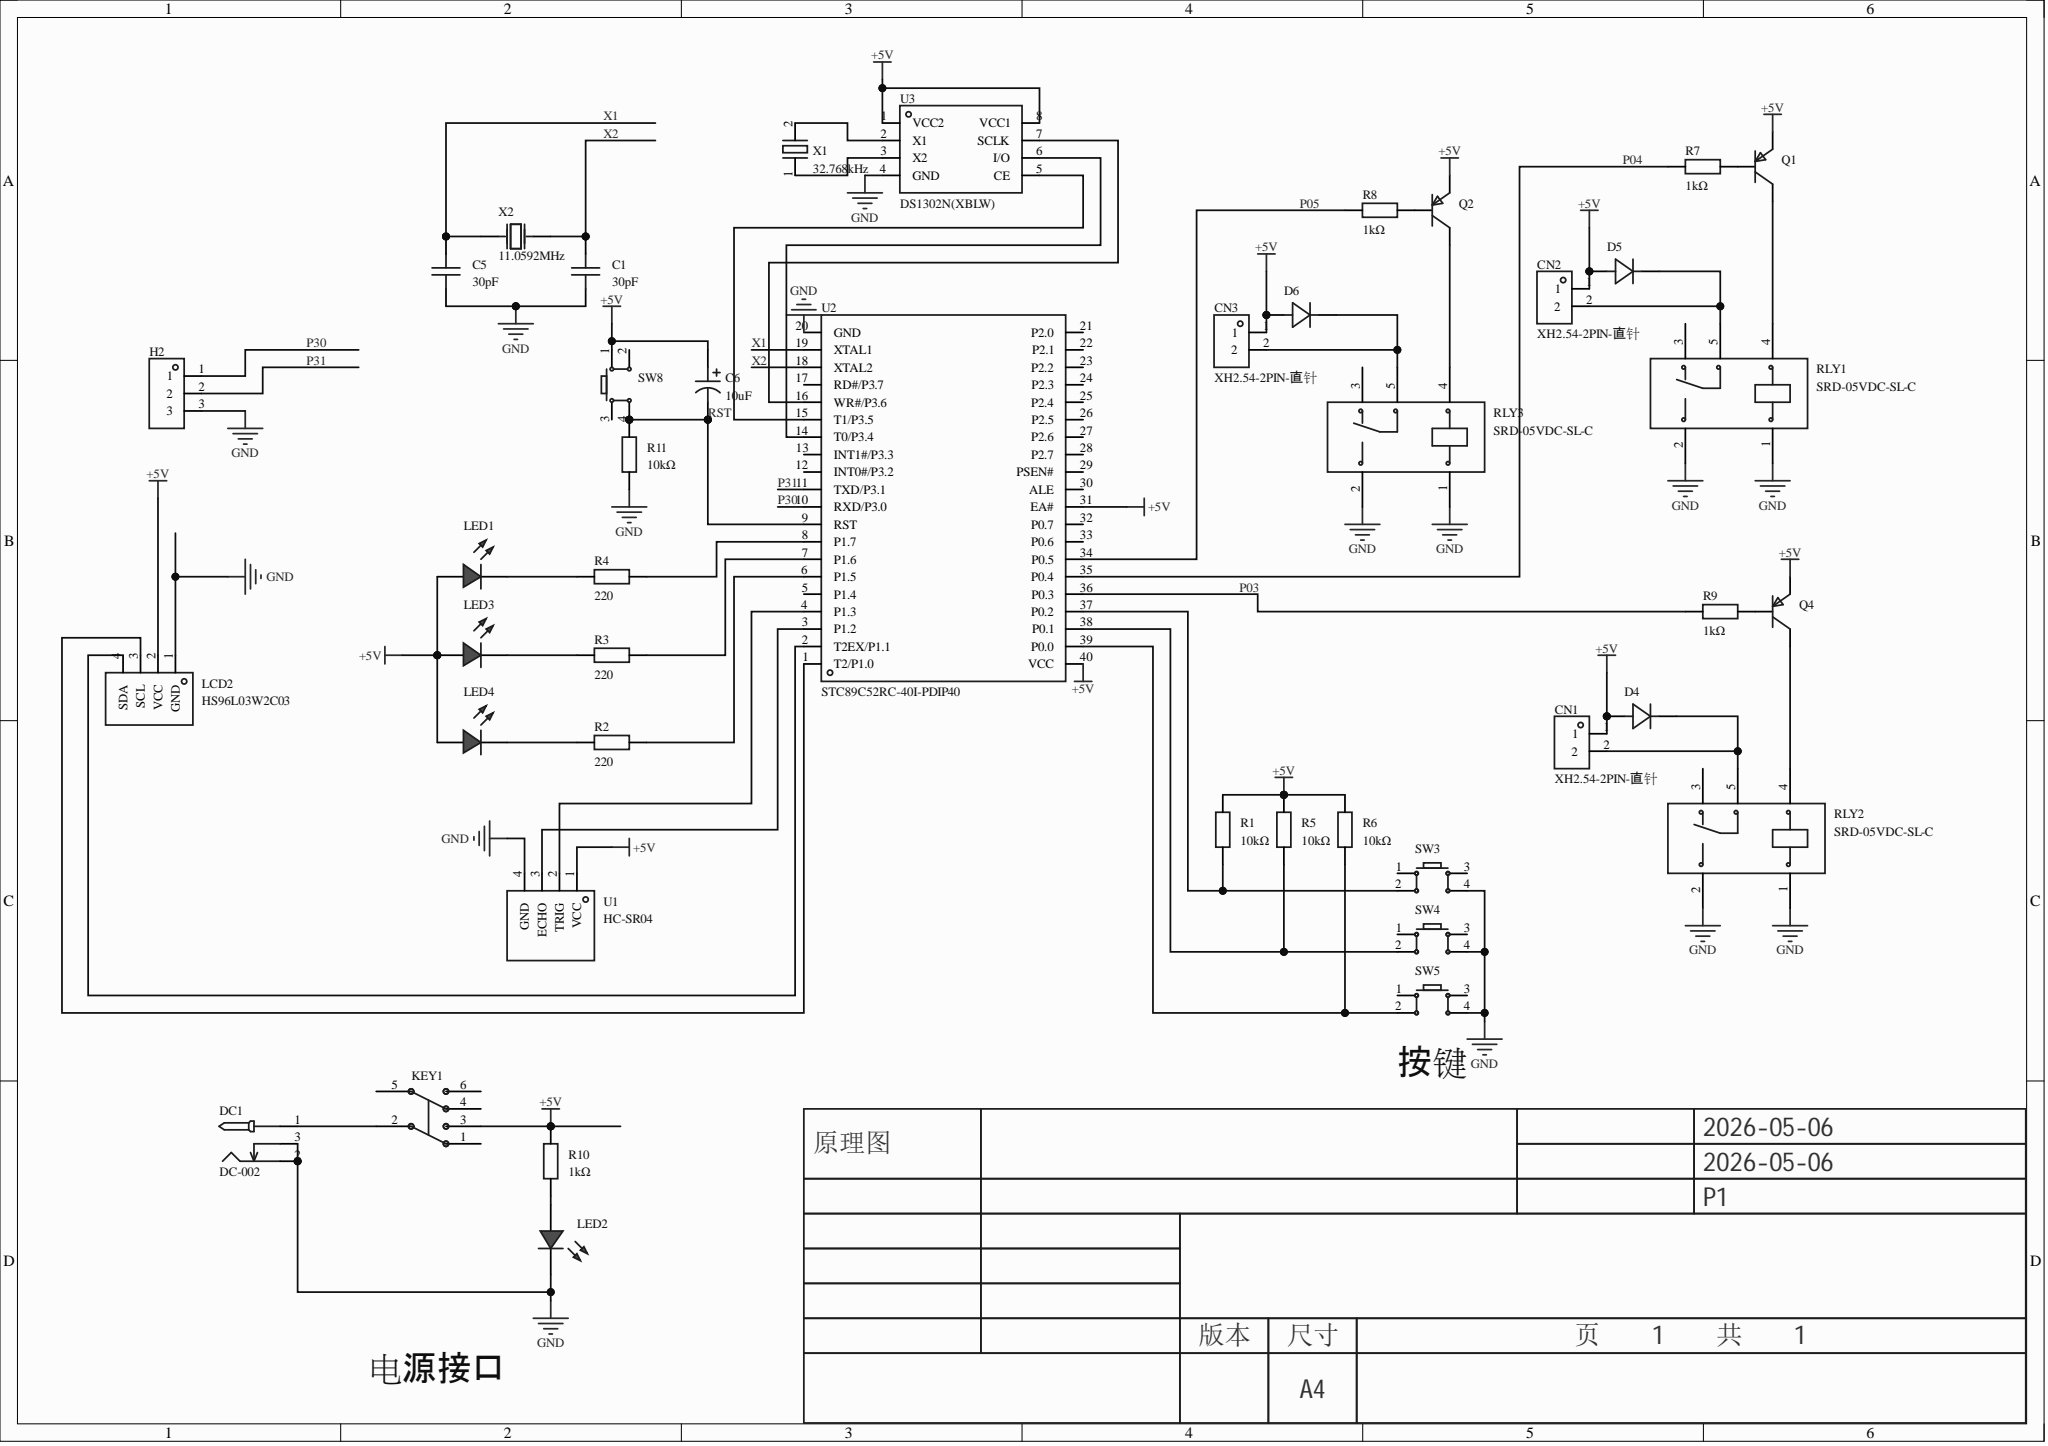Circuit board | Altium Designer | 43 parts | 39 nets
Bill of materials:
Comment,Description,Designator,Footprint,LibRef,Quantity
"30pF","","C1, C5","CAP-TH_L3.8-W2.5-P2.54-D0.50","C315C300K3G5TA7301","2"
"10uF","","C6","CAP-TH_BD5.0-P2.00-D0.8-FD-10UF50VC110GL","10UF50VC110GL","1"
"XH2.54-2PIN-直针","","CN1, CN2, CN3","CONN-TH_XH2.54-2P","XH2.54-2PIN-直针","3"
"","","D4, D5, D6","DO_1N4007","D_1N4007A","3"
"DC-002","","DC1","DC-IN-TH_DC-3510","DC-002","1"
"","","H2","HDR-TH_3P-P2.54-V-M","HDR-M_2.54_1x3P","1"
"无自锁开关 8.5×8.5 无声","","KEY1","SW-TH_6P-L8.5-W8.5-P2.54","无自锁开关 8.5×8.5 无声","1"
"HS96L03W2C03","","LCD2","OLED-TH_L27.8-W27.2-P2.54_C9900033791","HS96L03W2C03","1"
"","","LED1, LED2, LED3, LED4","LED_TH-3mm","LED_TH-R_3mm","4"
"","","Q1, Q2, Q4","S8550P_TO-92","S8550_TO_PNP","3"
"10kΩ","","R1, R5, R6, R11","Res_1/8W","Res_AXIAL-1/8W","4"
"220","","R2, R3, R4","R0603","Res_0603","3"
"1kΩ","","R7, R8, R9, R10","Res_1/8W","Res_AXIAL-1/8W","4"
"SRD-05VDC-SL-C","","RLY1, RLY2, RLY3","RELAY-TH_SRD-XXVDC-XL-C","SRD-05VDC-SL-C","3"
"","","SW3, SW4, SW5, SW8","SW-TH_4P-L6.0-W6.0-P4.50-LS6.5","Key_TH_6x6x6","4"
"HC-SR04","","U1","TH_HC-SR04V","HC-SR04","1"
"STC89C52RC-40I-PDIP40","","U2","DIP-40_L52.0-W13.7-P2.54-LS15.2-BL","STC89C52RC-40I-PDIP40","1"
"DS1302N(XBLW)","","U3","PDIP-8_L9.3-W6.4-P2.54-LS7.6-BL","DS1302N(XBLW)","1"
"32.768kHz","","X1","CRYSTAL-TH_BD1.4-P0.45-D0.2","AB15T-32.768KHZ","1"
"11.059MHz","","X2","OSC-TH_L11.1-W4.7-P4.88","9AC11059302060C3","1"
Netlist (Protel format):
[
C1
CAP-TH_L3.8-W2.5-P2.54-D0.50
30pF



]
[
C5
CAP-TH_L3.8-W2.5-P2.54-D0.50
30pF



]
[
C6
CAP-TH_BD5.0-P2.00-D0.8-FD-10UF50VC110GL
10uF



]
[
CN1
CONN-TH_XH2.54-2P
XH2.54-2PIN-直针



]
[
CN2
CONN-TH_XH2.54-2P
XH2.54-2PIN-直针



]
[
CN3
CONN-TH_XH2.54-2P
XH2.54-2PIN-直针



]
[
D4
DO_1N4007




]
[
D5
DO_1N4007




]
[
D6
DO_1N4007




]
[
DC1
DC-IN-TH_DC-3510
DC-002



]
[
H2
HDR-TH_3P-P2.54-V-M




]
[
KEY1
SW-TH_6P-L8.5-W8.5-P2.54
无自锁开关 8.5×8.5 无声



]
[
LCD2
OLED-TH_L27.8-W27.2-P2.54_C9900033791
HS96L03W2C03



]
[
LED1
LED_TH-3mm




]
[
LED2
LED_TH-3mm




]
[
LED3
LED_TH-3mm




]
[
LED4
LED_TH-3mm




]
[
Q1
S8550P_TO-92




]
[
Q2
S8550P_TO-92




]
[
Q4
S8550P_TO-92




]
[
R1
Res_1/8W
10kΩ



]
[
R2
R0603
220



]
[
R3
R0603
220



]
[
R4
R0603
220



]
[
R5
Res_1/8W
10kΩ



]
[
R6
Res_1/8W
10kΩ



]
[
R7
Res_1/8W
1kΩ



]
[
R8
Res_1/8W
1kΩ



]
[
R9
Res_1/8W
1kΩ



]
[
R10
Res_1/8W
1kΩ



]
[
R11
Res_1/8W
10kΩ



]
[
RLY1
RELAY-TH_SRD-XXVDC-XL-C
SRD-05VDC-SL-C



]
[
RLY2
RELAY-TH_SRD-XXVDC-XL-C
SRD-05VDC-SL-C



]
[
RLY3
RELAY-TH_SRD-XXVDC-XL-C
SRD-05VDC-SL-C



]
[
SW3
SW-TH_4P-L6.0-W6.0-P4.50-LS6.5




]
[
SW4
SW-TH_4P-L6.0-W6.0-P4.50-LS6.5




]
[
SW5
SW-TH_4P-L6.0-W6.0-P4.50-LS6.5




]
[
SW8
SW-TH_4P-L6.0-W6.0-P4.50-LS6.5




]
[
U1
TH_HC-SR04V
HC-SR04



]
[
U2
DIP-40_L52.0-W13.7-P2.54-LS15.2-BL
STC89C52RC-40I-PDIP40



]
[
U3
PDIP-8_L9.3-W6.4-P2.54-LS7.6-BL
DS1302N(XBLW)



]
[
X1
CRYSTAL-TH_BD1.4-P0.45-D0.2
32.768kHz



]
[
X2
OSC-TH_L11.1-W4.7-P4.88
11.0592MHz



]
(
X2
C1-2
U2-18
X2-2
)
(
X1
C5-2
U2-19
X2-1
)
(
RST
C6-2
R11-2
SW8-4
U2-9
)
(
P31
H2-2
U2-11
)
(
P30
H2-1
U2-10
)
(
P05
R8-2
U2-34
)
(
P04
R7-2
U2-35
)
(
P03
R9-2
U2-36
)
(
NetU3_3
U3-3
X1-1
)
(
NetU3_2
U3-2
X1-2
)
(
NetU2_16
U2-16
U3-7
)
(
NetU2_15
U2-15
U3-5
)
(
NetU2_14
U2-14
U3-6
)
(
NetU1_3
U1-3
U2-3
)
(
NetU1_2
U1-2
U2-4
)
(
NetR6_1
R6-1
SW5-2
U2-39
)
(
NetR5_1
R5-1
SW4-2
U2-38
)
(
NetR4_2
R4-2
U2-8
)
(
NetR3_2
R3-2
U2-7
)
(
NetR2_2
R2-2
U2-6
)
(
NetR1_1
R1-1
SW3-2
U2-37
)
(
NetQ4_3
Q4-3
RLY2-4
)
(
NetQ4_2
Q4-2
R9-1
)
(
NetQ2_3
Q2-3
RLY3-4
)
(
NetQ2_2
Q2-2
R8-1
)
(
NetQ1_3
Q1-3
RLY1-4
)
(
NetQ1_2
Q1-2
R7-1
)
(
NetLED4_2
LED4-2
R2-1
)
(
NetLED3_2
LED3-2
R3-1
)
(
NetLED2_1
LED2-1
R10-1
)
(
NetLED1_2
LED1-2
R4-1
)
(
NetLCD2_4
LCD2-4
U2-2
)
(
NetLCD2_3
LCD2-3
U2-1
)
(
NetDC1_1
DC1-1
KEY1-2
)
(
NetCN3_2
CN3-2
D6-1
RLY3-5
)
(
NetCN2_2
CN2-2
D5-1
RLY1-5
)
(
NetCN1_2
CN1-2
D4-1
RLY2-5
)
(
GND
C1-1
C5-1
DC1-2
DC1-3
H2-3
LCD2-1
LED2-2
R11-1
RLY1-1
RLY1-2
RLY2-1
RLY2-2
RLY3-1
RLY3-2
SW3-4
SW4-4
SW5-4
U1-4
U2-20
U3-4
)
(
+5V
C6-1
CN1-1
CN2-1
CN3-1
D4-2
D5-2
D6-2
KEY1-3
LCD2-2
LED1-1
LED3-1
LED4-1
Q1-1
Q2-1
Q4-1
R1-2
R5-2
R6-2
R10-2
SW8-1
U1-1
U2-31
U2-40
U3-1
U3-8
)